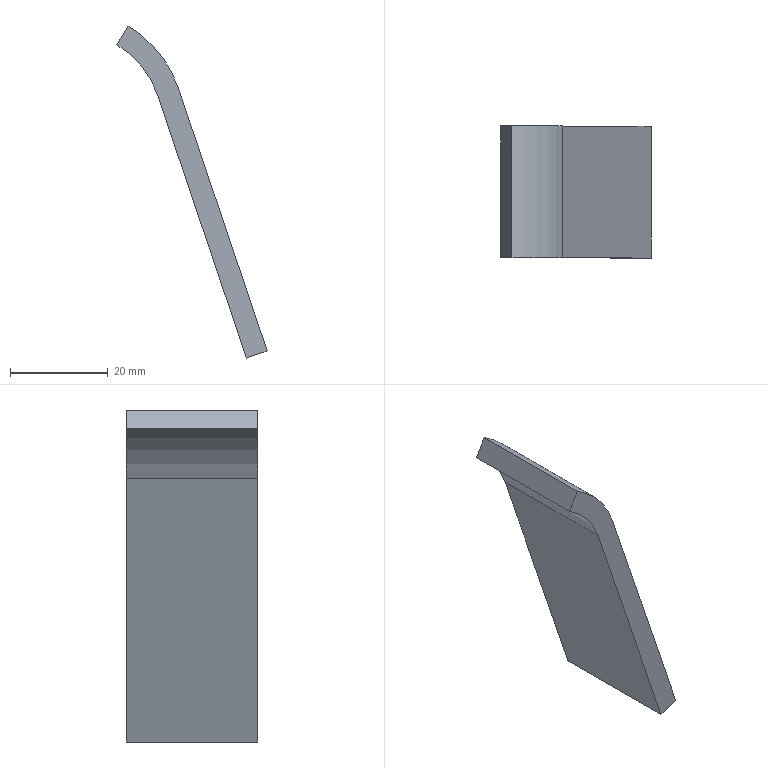Part | STEP file | 2026.6.15-Main Assembly图.sldasm-Part-255 | 1 solid | 8 faces | box 30.802 x 27 x 68.097 mm | volume 8755 mm3 | plane 6 | cylinder 2 | commonest cylinder face diameters 37.5 x1 46.5 x1
STEP:
#1=CARTESIAN_POINT('',(-1472.365,1437.764,3269.382));
#2=VERTEX_POINT('',#1);
#3=CARTESIAN_POINT('',(-1490.611,1437.764,3323.412));
#4=VERTEX_POINT('',#3);
#5=CARTESIAN_POINT('',(-1490.611,1437.764,3323.412));
#6=DIRECTION('',(-0.3199,0.,0.9474));
#7=VECTOR('',#6,1000.);
#8=LINE('',#5,#7);
#9=EDGE_CURVE('',#2,#4,#8,.T.);
#10=ORIENTED_EDGE('',*,*,#9,.F.);
#11=CARTESIAN_POINT('',(-1472.365,1410.764,3269.382));
#12=VERTEX_POINT('',#11);
#13=CARTESIAN_POINT('',(-1472.365,1437.764,3269.382));
#14=DIRECTION('',(0.,1.,0.));
#15=VECTOR('',#14,1000.);
#16=LINE('',#13,#15);
#17=EDGE_CURVE('',#12,#2,#16,.T.);
#18=ORIENTED_EDGE('',*,*,#17,.F.);
#19=CARTESIAN_POINT('',(-1490.611,1410.764,3323.412));
#20=VERTEX_POINT('',#19);
#21=CARTESIAN_POINT('',(-1490.611,1410.764,3323.412));
#22=DIRECTION('',(-0.3199,0.,0.9474));
#23=VECTOR('',#22,1000.);
#24=LINE('',#21,#23);
#25=EDGE_CURVE('',#12,#20,#24,.T.);
#26=ORIENTED_EDGE('',*,*,#25,.T.);
#27=CARTESIAN_POINT('',(-1490.611,1437.764,3323.412));
#28=DIRECTION('',(0.,1.,0.));
#29=VECTOR('',#28,1000.);
#30=LINE('',#27,#29);
#31=EDGE_CURVE('',#20,#4,#30,.T.);
#32=ORIENTED_EDGE('',*,*,#31,.T.);
#33=EDGE_LOOP('',(#10,#18,#26,#32));
#34=FACE_OUTER_BOUND('',#33,.T.);
#35=CARTESIAN_POINT('',(-1472.365,1437.764,3269.382));
#36=DIRECTION('',(-0.9474,0.,-0.3199));
#37=DIRECTION('',(0.,1.,0.));
#38=AXIS2_PLACEMENT_3D('',#35,#36,#37);
#39=PLANE('',#38);
#40=ADVANCED_FACE('',(#34),#39,.T.);
#41=CARTESIAN_POINT('',(-1498.904,1437.764,3333.595));
#42=VERTEX_POINT('',#41);
#43=CARTESIAN_POINT('',(-1498.904,1410.764,3333.595));
#44=VERTEX_POINT('',#43);
#45=CARTESIAN_POINT('',(-1498.904,1437.764,3333.595));
#46=DIRECTION('',(0.,-1.,0.));
#47=VECTOR('',#46,1000.);
#48=LINE('',#45,#47);
#49=EDGE_CURVE('',#42,#44,#48,.T.);
#50=ORIENTED_EDGE('',*,*,#49,.F.);
#51=CARTESIAN_POINT('',(-1508.375,1437.764,3317.413));
#52=DIRECTION('',(0.,-1.,0.));
#53=DIRECTION('',(0.9474,0.,0.3199));
#54=AXIS2_PLACEMENT_3D('',#51,#52,#53);
#55=CIRCLE('',#54,18.75);
#56=EDGE_CURVE('',#4,#42,#55,.T.);
#57=ORIENTED_EDGE('',*,*,#56,.F.);
#58=ORIENTED_EDGE('',*,*,#31,.F.);
#59=CARTESIAN_POINT('',(-1508.375,1410.764,3317.413));
#60=DIRECTION('',(0.,-1.,0.));
#61=DIRECTION('',(0.9474,0.,0.3199));
#62=AXIS2_PLACEMENT_3D('',#59,#60,#61);
#63=CIRCLE('',#62,18.75);
#64=EDGE_CURVE('',#20,#44,#63,.T.);
#65=ORIENTED_EDGE('',*,*,#64,.T.);
#66=EDGE_LOOP('',(#50,#57,#58,#65));
#67=FACE_OUTER_BOUND('',#66,.T.);
#68=CARTESIAN_POINT('',(-1508.375,1437.764,3317.413));
#69=DIRECTION('',(0.,-1.,0.));
#70=DIRECTION('',(-0.9474,0.,-0.3199));
#71=AXIS2_PLACEMENT_3D('',#68,#69,#70);
#72=CYLINDRICAL_SURFACE('',#71,18.75);
#73=ADVANCED_FACE('',(#67),#72,.F.);
#74=CARTESIAN_POINT('',(-1496.631,1437.764,3337.479));
#75=VERTEX_POINT('',#74);
#76=CARTESIAN_POINT('',(-1498.904,1437.764,3333.595));
#77=DIRECTION('',(0.5051,0.,0.863));
#78=VECTOR('',#77,1000.);
#79=LINE('',#76,#78);
#80=EDGE_CURVE('',#42,#75,#79,.T.);
#81=ORIENTED_EDGE('',*,*,#80,.F.);
#82=ORIENTED_EDGE('',*,*,#49,.T.);
#83=CARTESIAN_POINT('',(-1496.631,1410.764,3337.479));
#84=VERTEX_POINT('',#83);
#85=CARTESIAN_POINT('',(-1498.904,1410.764,3333.595));
#86=DIRECTION('',(0.5051,0.,0.863));
#87=VECTOR('',#86,1000.);
#88=LINE('',#85,#87);
#89=EDGE_CURVE('',#44,#84,#88,.T.);
#90=ORIENTED_EDGE('',*,*,#89,.T.);
#91=CARTESIAN_POINT('',(-1496.631,1437.764,3337.479));
#92=DIRECTION('',(0.,-1.,0.));
#93=VECTOR('',#92,1000.);
#94=LINE('',#91,#93);
#95=EDGE_CURVE('',#75,#84,#94,.T.);
#96=ORIENTED_EDGE('',*,*,#95,.F.);
#97=EDGE_LOOP('',(#81,#82,#90,#96));
#98=FACE_OUTER_BOUND('',#97,.T.);
#99=CARTESIAN_POINT('',(-1496.631,1437.764,3337.479));
#100=DIRECTION('',(-0.863,0.,0.5051));
#101=DIRECTION('',(0.,1.,0.));
#102=AXIS2_PLACEMENT_3D('',#99,#100,#101);
#103=PLANE('',#102);
#104=ADVANCED_FACE('',(#98),#103,.T.);
#105=CARTESIAN_POINT('',(-1486.347,1437.764,3324.852));
#106=VERTEX_POINT('',#105);
#107=CARTESIAN_POINT('',(-1508.375,1437.764,3317.413));
#108=DIRECTION('',(0.,1.,0.));
#109=DIRECTION('',(0.9474,0.,0.3199));
#110=AXIS2_PLACEMENT_3D('',#107,#108,#109);
#111=CIRCLE('',#110,23.25);
#112=EDGE_CURVE('',#75,#106,#111,.T.);
#113=ORIENTED_EDGE('',*,*,#112,.F.);
#114=ORIENTED_EDGE('',*,*,#95,.T.);
#115=CARTESIAN_POINT('',(-1486.347,1410.764,3324.852));
#116=VERTEX_POINT('',#115);
#117=CARTESIAN_POINT('',(-1508.375,1410.764,3317.413));
#118=DIRECTION('',(0.,1.,0.));
#119=DIRECTION('',(0.9474,0.,0.3199));
#120=AXIS2_PLACEMENT_3D('',#117,#118,#119);
#121=CIRCLE('',#120,23.25);
#122=EDGE_CURVE('',#84,#116,#121,.T.);
#123=ORIENTED_EDGE('',*,*,#122,.T.);
#124=CARTESIAN_POINT('',(-1486.347,1437.764,3324.852));
#125=DIRECTION('',(0.,1.,0.));
#126=VECTOR('',#125,1000.);
#127=LINE('',#124,#126);
#128=EDGE_CURVE('',#116,#106,#127,.T.);
#129=ORIENTED_EDGE('',*,*,#128,.T.);
#130=EDGE_LOOP('',(#113,#114,#123,#129));
#131=FACE_OUTER_BOUND('',#130,.T.);
#132=CARTESIAN_POINT('',(-1508.375,1437.764,3317.413));
#133=DIRECTION('',(0.,-1.,0.));
#134=DIRECTION('',(-0.9474,0.,-0.3199));
#135=AXIS2_PLACEMENT_3D('',#132,#133,#134);
#136=CYLINDRICAL_SURFACE('',#135,23.25);
#137=ADVANCED_FACE('',(#131),#136,.T.);
#138=ORIENTED_EDGE('',*,*,#80,.T.);
#139=ORIENTED_EDGE('',*,*,#112,.T.);
#140=CARTESIAN_POINT('',(-1468.101,1437.764,3270.822));
#141=VERTEX_POINT('',#140);
#142=CARTESIAN_POINT('',(-1468.101,1437.764,3270.822));
#143=DIRECTION('',(0.3199,0.,-0.9474));
#144=VECTOR('',#143,1000.);
#145=LINE('',#142,#144);
#146=EDGE_CURVE('',#106,#141,#145,.T.);
#147=ORIENTED_EDGE('',*,*,#146,.T.);
#148=CARTESIAN_POINT('',(-1472.365,1437.764,3269.382));
#149=DIRECTION('',(0.9474,0.,0.3199));
#150=VECTOR('',#149,1000.);
#151=LINE('',#148,#150);
#152=EDGE_CURVE('',#2,#141,#151,.T.);
#153=ORIENTED_EDGE('',*,*,#152,.F.);
#154=ORIENTED_EDGE('',*,*,#9,.T.);
#155=ORIENTED_EDGE('',*,*,#56,.T.);
#156=EDGE_LOOP('',(#138,#139,#147,#153,#154,#155));
#157=FACE_OUTER_BOUND('',#156,.T.);
#158=CARTESIAN_POINT('',(-1508.375,1437.764,3317.413));
#159=DIRECTION('',(0.,1.,0.));
#160=DIRECTION('',(1.,0.,0.));
#161=AXIS2_PLACEMENT_3D('',#158,#159,#160);
#162=PLANE('',#161);
#163=ADVANCED_FACE('',(#157),#162,.T.);
#164=ORIENTED_EDGE('',*,*,#152,.T.);
#165=CARTESIAN_POINT('',(-1468.101,1410.764,3270.822));
#166=VERTEX_POINT('',#165);
#167=CARTESIAN_POINT('',(-1468.101,1437.764,3270.822));
#168=DIRECTION('',(0.,-1.,0.));
#169=VECTOR('',#168,1000.);
#170=LINE('',#167,#169);
#171=EDGE_CURVE('',#141,#166,#170,.T.);
#172=ORIENTED_EDGE('',*,*,#171,.T.);
#173=CARTESIAN_POINT('',(-1490.129,1410.764,3263.383));
#174=DIRECTION('',(-0.9474,0.,-0.3199));
#175=VECTOR('',#174,1000.);
#176=LINE('',#173,#175);
#177=EDGE_CURVE('',#166,#12,#176,.T.);
#178=ORIENTED_EDGE('',*,*,#177,.T.);
#179=ORIENTED_EDGE('',*,*,#17,.T.);
#180=EDGE_LOOP('',(#164,#172,#178,#179));
#181=FACE_OUTER_BOUND('',#180,.T.);
#182=CARTESIAN_POINT('',(-1472.365,1437.764,3269.382));
#183=DIRECTION('',(0.3199,0.,-0.9474));
#184=DIRECTION('',(0.,-1.,0.));
#185=AXIS2_PLACEMENT_3D('',#182,#183,#184);
#186=PLANE('',#185);
#187=ADVANCED_FACE('',(#181),#186,.T.);
#188=ORIENTED_EDGE('',*,*,#122,.F.);
#189=ORIENTED_EDGE('',*,*,#89,.F.);
#190=ORIENTED_EDGE('',*,*,#64,.F.);
#191=ORIENTED_EDGE('',*,*,#25,.F.);
#192=ORIENTED_EDGE('',*,*,#177,.F.);
#193=CARTESIAN_POINT('',(-1468.101,1410.764,3270.822));
#194=DIRECTION('',(-0.3199,0.,0.9474));
#195=VECTOR('',#194,1000.);
#196=LINE('',#193,#195);
#197=EDGE_CURVE('',#166,#116,#196,.T.);
#198=ORIENTED_EDGE('',*,*,#197,.T.);
#199=EDGE_LOOP('',(#188,#189,#190,#191,#192,#198));
#200=FACE_OUTER_BOUND('',#199,.T.);
#201=CARTESIAN_POINT('',(-1508.375,1410.764,3317.413));
#202=DIRECTION('',(0.,1.,0.));
#203=DIRECTION('',(1.,0.,0.));
#204=AXIS2_PLACEMENT_3D('',#201,#202,#203);
#205=PLANE('',#204);
#206=ADVANCED_FACE('',(#200),#205,.F.);
#207=ORIENTED_EDGE('',*,*,#171,.F.);
#208=ORIENTED_EDGE('',*,*,#146,.F.);
#209=ORIENTED_EDGE('',*,*,#128,.F.);
#210=ORIENTED_EDGE('',*,*,#197,.F.);
#211=EDGE_LOOP('',(#207,#208,#209,#210));
#212=FACE_OUTER_BOUND('',#211,.T.);
#213=CARTESIAN_POINT('',(-1468.101,1437.764,3270.822));
#214=DIRECTION('',(-0.9474,0.,-0.3199));
#215=DIRECTION('',(0.,1.,0.));
#216=AXIS2_PLACEMENT_3D('',#213,#214,#215);
#217=PLANE('',#216);
#218=ADVANCED_FACE('',(#212),#217,.F.);
#219=CLOSED_SHELL('',(#40,#73,#104,#137,#163,#187,#206,#218));
#220=MANIFOLD_SOLID_BREP('',#219);
#221=CARTESIAN_POINT('',(0.,0.,0.));
#222=DIRECTION('',(0.,0.,1.));
#223=DIRECTION('',(1.,0.,0.));
#224=AXIS2_PLACEMENT_3D('',#221,#222,#223);
#225=(LENGTH_UNIT()NAMED_UNIT(*)SI_UNIT(.MILLI.,.METRE.));
#226=UNCERTAINTY_MEASURE_WITH_UNIT(LENGTH_MEASURE(0.00001),#225,'','');
#227=(NAMED_UNIT(*)PLANE_ANGLE_UNIT()SI_UNIT($,.RADIAN.));
#228=(NAMED_UNIT(*)SI_UNIT($,.STERADIAN.)SOLID_ANGLE_UNIT());
#229=(GEOMETRIC_REPRESENTATION_CONTEXT(3)GLOBAL_UNCERTAINTY_ASSIGNED_CONTEXT((#226))GLOBAL_UNIT_ASSIGNED_CONTEXT((#225,#227,#228))REPRESENTATION_CONTEXT('',''));
#230=ADVANCED_BREP_SHAPE_REPRESENTATION('',(#220,#224),#229);